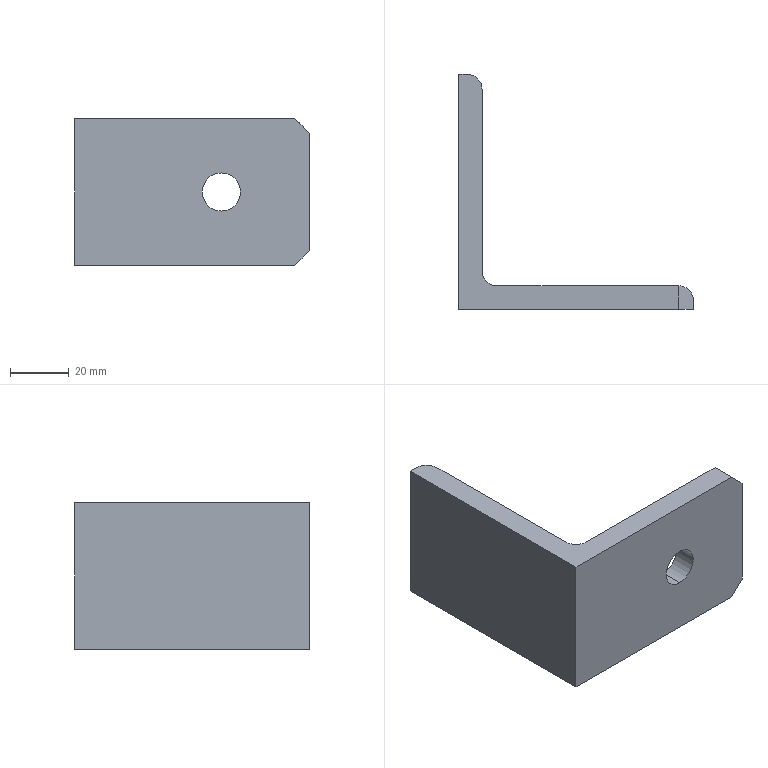Part | SolidWorks | features Fillet 3, Chamfer 1, Extrusion 1, ICE 1 | 1 solid | 15 faces | box 80 x 80 x 50 mm | volume 59312 mm3 | plane 10 | cylinder 5 | commonest cylinder face diameters 10 x3 13 x2
STEP:
#1=CARTESIAN_POINT('',(50.,-80.,18.5));
#2=VERTEX_POINT('',#1);
#3=CARTESIAN_POINT('',(50.,-80.,31.5));
#4=VERTEX_POINT('',#3);
#5=CARTESIAN_POINT('',(50.,-80.,25.));
#6=DIRECTION('',(0.,1.,0.));
#7=DIRECTION('',(0.,0.,1.));
#8=AXIS2_PLACEMENT_3D('',#5,#6,#7);
#9=CIRCLE('',#8,6.5);
#10=EDGE_CURVE('',#2,#4,#9,.T.);
#11=ORIENTED_EDGE('',*,*,#10,.F.);
#12=CARTESIAN_POINT('',(50.,-72.,18.5));
#13=VERTEX_POINT('',#12);
#14=CARTESIAN_POINT('',(50.,-122.,18.5));
#15=DIRECTION('',(0.,1.,0.));
#16=VECTOR('',#15,1000.);
#17=LINE('',#14,#16);
#18=EDGE_CURVE('',#2,#13,#17,.T.);
#19=ORIENTED_EDGE('',*,*,#18,.T.);
#20=CARTESIAN_POINT('',(50.,-72.,31.5));
#21=VERTEX_POINT('',#20);
#22=CARTESIAN_POINT('',(50.,-72.,25.));
#23=DIRECTION('',(0.,1.,0.));
#24=DIRECTION('',(0.,0.,1.));
#25=AXIS2_PLACEMENT_3D('',#22,#23,#24);
#26=CIRCLE('',#25,6.5);
#27=EDGE_CURVE('',#13,#21,#26,.T.);
#28=ORIENTED_EDGE('',*,*,#27,.T.);
#29=CARTESIAN_POINT('',(50.,-122.,31.5));
#30=DIRECTION('',(0.,1.,0.));
#31=VECTOR('',#30,1000.);
#32=LINE('',#29,#31);
#33=EDGE_CURVE('',#4,#21,#32,.T.);
#34=ORIENTED_EDGE('',*,*,#33,.F.);
#35=EDGE_LOOP('',(#11,#19,#28,#34));
#36=FACE_OUTER_BOUND('',#35,.T.);
#37=CARTESIAN_POINT('',(50.,-122.,25.));
#38=DIRECTION('',(0.,1.,0.));
#39=DIRECTION('',(0.,0.,1.));
#40=AXIS2_PLACEMENT_3D('',#37,#38,#39);
#41=CYLINDRICAL_SURFACE('',#40,6.5);
#42=ADVANCED_FACE('',(#36),#41,.F.);
#43=CARTESIAN_POINT('',(50.,-72.,25.));
#44=DIRECTION('',(0.,1.,0.));
#45=DIRECTION('',(0.,0.,1.));
#46=AXIS2_PLACEMENT_3D('',#43,#44,#45);
#47=CIRCLE('',#46,6.5);
#48=EDGE_CURVE('',#21,#13,#47,.T.);
#49=ORIENTED_EDGE('',*,*,#48,.F.);
#50=ORIENTED_EDGE('',*,*,#27,.F.);
#51=EDGE_LOOP('',(#49,#50));
#52=FACE_BOUND('',#51,.T.);
#53=CARTESIAN_POINT('',(13.,-72.,50.));
#54=VERTEX_POINT('',#53);
#55=CARTESIAN_POINT('',(75.,-72.,50.));
#56=VERTEX_POINT('',#55);
#57=CARTESIAN_POINT('',(8.,-72.,50.));
#58=DIRECTION('',(1.,0.,0.));
#59=VECTOR('',#58,1000.);
#60=LINE('',#57,#59);
#61=EDGE_CURVE('',#54,#56,#60,.T.);
#62=ORIENTED_EDGE('',*,*,#61,.T.);
#63=CARTESIAN_POINT('',(75.,-72.,0.));
#64=VERTEX_POINT('',#63);
#65=CARTESIAN_POINT('',(75.,-72.,50.));
#66=DIRECTION('',(0.,0.,-1.));
#67=VECTOR('',#66,1000.);
#68=LINE('',#65,#67);
#69=EDGE_CURVE('',#56,#64,#68,.T.);
#70=ORIENTED_EDGE('',*,*,#69,.T.);
#71=CARTESIAN_POINT('',(13.,-72.,0.));
#72=VERTEX_POINT('',#71);
#73=CARTESIAN_POINT('',(8.,-72.,0.));
#74=DIRECTION('',(1.,0.,0.));
#75=VECTOR('',#74,1000.);
#76=LINE('',#73,#75);
#77=EDGE_CURVE('',#72,#64,#76,.T.);
#78=ORIENTED_EDGE('',*,*,#77,.F.);
#79=CARTESIAN_POINT('',(13.,-72.,50.));
#80=DIRECTION('',(0.,0.,1.));
#81=VECTOR('',#80,1000.);
#82=LINE('',#79,#81);
#83=EDGE_CURVE('',#72,#54,#82,.T.);
#84=ORIENTED_EDGE('',*,*,#83,.T.);
#85=EDGE_LOOP('',(#62,#70,#78,#84));
#86=FACE_OUTER_BOUND('',#85,.T.);
#87=CARTESIAN_POINT('',(8.,-72.,50.));
#88=DIRECTION('',(0.,1.,0.));
#89=DIRECTION('',(0.,0.,1.));
#90=AXIS2_PLACEMENT_3D('',#87,#88,#89);
#91=PLANE('',#90);
#92=ADVANCED_FACE('',(#52,#86),#91,.T.);
#93=CARTESIAN_POINT('',(8.,-5.,0.));
#94=VERTEX_POINT('',#93);
#95=CARTESIAN_POINT('',(8.,-67.,0.));
#96=VERTEX_POINT('',#95);
#97=CARTESIAN_POINT('',(8.,0.,0.));
#98=DIRECTION('',(0.,-1.,0.));
#99=VECTOR('',#98,1000.);
#100=LINE('',#97,#99);
#101=EDGE_CURVE('',#94,#96,#100,.T.);
#102=ORIENTED_EDGE('',*,*,#101,.F.);
#103=CARTESIAN_POINT('',(8.,-5.,50.));
#104=VERTEX_POINT('',#103);
#105=CARTESIAN_POINT('',(8.,-5.,50.));
#106=DIRECTION('',(0.,0.,1.));
#107=VECTOR('',#106,1000.);
#108=LINE('',#105,#107);
#109=EDGE_CURVE('',#94,#104,#108,.T.);
#110=ORIENTED_EDGE('',*,*,#109,.T.);
#111=CARTESIAN_POINT('',(8.,-67.,50.));
#112=VERTEX_POINT('',#111);
#113=CARTESIAN_POINT('',(8.,0.,50.));
#114=DIRECTION('',(0.,-1.,0.));
#115=VECTOR('',#114,1000.);
#116=LINE('',#113,#115);
#117=EDGE_CURVE('',#104,#112,#116,.T.);
#118=ORIENTED_EDGE('',*,*,#117,.T.);
#119=CARTESIAN_POINT('',(8.,-67.,0.));
#120=DIRECTION('',(0.,0.,-1.));
#121=VECTOR('',#120,1000.);
#122=LINE('',#119,#121);
#123=EDGE_CURVE('',#112,#96,#122,.T.);
#124=ORIENTED_EDGE('',*,*,#123,.T.);
#125=EDGE_LOOP('',(#102,#110,#118,#124));
#126=FACE_OUTER_BOUND('',#125,.T.);
#127=CARTESIAN_POINT('',(8.,0.,50.));
#128=DIRECTION('',(1.,0.,0.));
#129=DIRECTION('',(0.,0.,-1.));
#130=AXIS2_PLACEMENT_3D('',#127,#128,#129);
#131=PLANE('',#130);
#132=ADVANCED_FACE('',(#126),#131,.T.);
#133=CARTESIAN_POINT('',(3.,0.,50.));
#134=VERTEX_POINT('',#133);
#135=CARTESIAN_POINT('',(0.,0.,50.));
#136=VERTEX_POINT('',#135);
#137=CARTESIAN_POINT('',(8.,0.,50.));
#138=DIRECTION('',(-1.,0.,0.));
#139=VECTOR('',#138,1000.);
#140=LINE('',#137,#139);
#141=EDGE_CURVE('',#134,#136,#140,.T.);
#142=ORIENTED_EDGE('',*,*,#141,.F.);
#143=CARTESIAN_POINT('',(3.,0.,0.));
#144=VERTEX_POINT('',#143);
#145=CARTESIAN_POINT('',(3.,0.,0.));
#146=DIRECTION('',(0.,0.,-1.));
#147=VECTOR('',#146,1000.);
#148=LINE('',#145,#147);
#149=EDGE_CURVE('',#134,#144,#148,.T.);
#150=ORIENTED_EDGE('',*,*,#149,.T.);
#151=CARTESIAN_POINT('',(0.,0.,0.));
#152=VERTEX_POINT('',#151);
#153=CARTESIAN_POINT('',(8.,0.,0.));
#154=DIRECTION('',(-1.,0.,0.));
#155=VECTOR('',#154,1000.);
#156=LINE('',#153,#155);
#157=EDGE_CURVE('',#144,#152,#156,.T.);
#158=ORIENTED_EDGE('',*,*,#157,.T.);
#159=CARTESIAN_POINT('',(0.,0.,50.));
#160=DIRECTION('',(0.,0.,-1.));
#161=VECTOR('',#160,1000.);
#162=LINE('',#159,#161);
#163=EDGE_CURVE('',#136,#152,#162,.T.);
#164=ORIENTED_EDGE('',*,*,#163,.F.);
#165=EDGE_LOOP('',(#142,#150,#158,#164));
#166=FACE_OUTER_BOUND('',#165,.T.);
#167=CARTESIAN_POINT('',(8.,0.,50.));
#168=DIRECTION('',(0.,-1.,0.));
#169=DIRECTION('',(0.,0.,-1.));
#170=AXIS2_PLACEMENT_3D('',#167,#168,#169);
#171=PLANE('',#170);
#172=ADVANCED_FACE('',(#166),#171,.F.);
#173=CARTESIAN_POINT('',(0.,-80.,0.));
#174=VERTEX_POINT('',#173);
#175=CARTESIAN_POINT('',(0.,0.,0.));
#176=DIRECTION('',(0.,-1.,0.));
#177=VECTOR('',#176,1000.);
#178=LINE('',#175,#177);
#179=EDGE_CURVE('',#152,#174,#178,.T.);
#180=ORIENTED_EDGE('',*,*,#179,.T.);
#181=CARTESIAN_POINT('',(0.,-80.,50.));
#182=VERTEX_POINT('',#181);
#183=CARTESIAN_POINT('',(0.,-80.,50.));
#184=DIRECTION('',(0.,0.,-1.));
#185=VECTOR('',#184,1000.);
#186=LINE('',#183,#185);
#187=EDGE_CURVE('',#182,#174,#186,.T.);
#188=ORIENTED_EDGE('',*,*,#187,.F.);
#189=CARTESIAN_POINT('',(0.,0.,50.));
#190=DIRECTION('',(0.,-1.,0.));
#191=VECTOR('',#190,1000.);
#192=LINE('',#189,#191);
#193=EDGE_CURVE('',#136,#182,#192,.T.);
#194=ORIENTED_EDGE('',*,*,#193,.F.);
#195=ORIENTED_EDGE('',*,*,#163,.T.);
#196=EDGE_LOOP('',(#180,#188,#194,#195));
#197=FACE_OUTER_BOUND('',#196,.T.);
#198=CARTESIAN_POINT('',(0.,0.,50.));
#199=DIRECTION('',(1.,0.,0.));
#200=DIRECTION('',(0.,0.,-1.));
#201=AXIS2_PLACEMENT_3D('',#198,#199,#200);
#202=PLANE('',#201);
#203=ADVANCED_FACE('',(#197),#202,.F.);
#204=CARTESIAN_POINT('',(50.,-80.,25.));
#205=DIRECTION('',(0.,1.,0.));
#206=DIRECTION('',(0.,0.,1.));
#207=AXIS2_PLACEMENT_3D('',#204,#205,#206);
#208=CIRCLE('',#207,6.5);
#209=EDGE_CURVE('',#4,#2,#208,.T.);
#210=ORIENTED_EDGE('',*,*,#209,.T.);
#211=ORIENTED_EDGE('',*,*,#10,.T.);
#212=EDGE_LOOP('',(#210,#211));
#213=FACE_BOUND('',#212,.T.);
#214=CARTESIAN_POINT('',(75.,-80.,0.));
#215=VERTEX_POINT('',#214);
#216=CARTESIAN_POINT('',(0.,-80.,0.));
#217=DIRECTION('',(1.,0.,0.));
#218=VECTOR('',#217,1000.);
#219=LINE('',#216,#218);
#220=EDGE_CURVE('',#174,#215,#219,.T.);
#221=ORIENTED_EDGE('',*,*,#220,.T.);
#222=CARTESIAN_POINT('',(80.,-80.,5.));
#223=VERTEX_POINT('',#222);
#224=CARTESIAN_POINT('',(75.,-80.,0.));
#225=DIRECTION('',(0.7071,0.,0.7071));
#226=VECTOR('',#225,1000.);
#227=LINE('',#224,#226);
#228=EDGE_CURVE('',#215,#223,#227,.T.);
#229=ORIENTED_EDGE('',*,*,#228,.T.);
#230=CARTESIAN_POINT('',(80.,-80.,45.));
#231=VERTEX_POINT('',#230);
#232=CARTESIAN_POINT('',(80.,-80.,50.));
#233=DIRECTION('',(0.,0.,-1.));
#234=VECTOR('',#233,1000.);
#235=LINE('',#232,#234);
#236=EDGE_CURVE('',#231,#223,#235,.T.);
#237=ORIENTED_EDGE('',*,*,#236,.F.);
#238=CARTESIAN_POINT('',(75.,-80.,50.));
#239=VERTEX_POINT('',#238);
#240=CARTESIAN_POINT('',(80.,-80.,45.));
#241=DIRECTION('',(-0.7071,0.,0.7071));
#242=VECTOR('',#241,1000.);
#243=LINE('',#240,#242);
#244=EDGE_CURVE('',#231,#239,#243,.T.);
#245=ORIENTED_EDGE('',*,*,#244,.T.);
#246=CARTESIAN_POINT('',(0.,-80.,50.));
#247=DIRECTION('',(1.,0.,0.));
#248=VECTOR('',#247,1000.);
#249=LINE('',#246,#248);
#250=EDGE_CURVE('',#182,#239,#249,.T.);
#251=ORIENTED_EDGE('',*,*,#250,.F.);
#252=ORIENTED_EDGE('',*,*,#187,.T.);
#253=EDGE_LOOP('',(#221,#229,#237,#245,#251,#252));
#254=FACE_OUTER_BOUND('',#253,.T.);
#255=CARTESIAN_POINT('',(0.,-80.,50.));
#256=DIRECTION('',(0.,1.,0.));
#257=DIRECTION('',(0.,0.,1.));
#258=AXIS2_PLACEMENT_3D('',#255,#256,#257);
#259=PLANE('',#258);
#260=ADVANCED_FACE('',(#213,#254),#259,.F.);
#261=CARTESIAN_POINT('',(80.,-77.,5.));
#262=VERTEX_POINT('',#261);
#263=CARTESIAN_POINT('',(80.,-72.,5.));
#264=DIRECTION('',(0.,1.,0.));
#265=VECTOR('',#264,1000.);
#266=LINE('',#263,#265);
#267=EDGE_CURVE('',#223,#262,#266,.T.);
#268=ORIENTED_EDGE('',*,*,#267,.T.);
#269=CARTESIAN_POINT('',(80.,-77.,45.));
#270=VERTEX_POINT('',#269);
#271=CARTESIAN_POINT('',(80.,-77.,50.));
#272=DIRECTION('',(0.,0.,1.));
#273=VECTOR('',#272,1000.);
#274=LINE('',#271,#273);
#275=EDGE_CURVE('',#262,#270,#274,.T.);
#276=ORIENTED_EDGE('',*,*,#275,.T.);
#277=CARTESIAN_POINT('',(80.,-80.,45.));
#278=DIRECTION('',(0.,-1.,0.));
#279=VECTOR('',#278,1000.);
#280=LINE('',#277,#279);
#281=EDGE_CURVE('',#270,#231,#280,.T.);
#282=ORIENTED_EDGE('',*,*,#281,.T.);
#283=ORIENTED_EDGE('',*,*,#236,.T.);
#284=EDGE_LOOP('',(#268,#276,#282,#283));
#285=FACE_OUTER_BOUND('',#284,.T.);
#286=CARTESIAN_POINT('',(80.,-72.,50.));
#287=DIRECTION('',(1.,0.,0.));
#288=DIRECTION('',(0.,0.,-1.));
#289=AXIS2_PLACEMENT_3D('',#286,#287,#288);
#290=PLANE('',#289);
#291=ADVANCED_FACE('',(#285),#290,.T.);
#292=ORIENTED_EDGE('',*,*,#250,.T.);
#293=CARTESIAN_POINT('',(75.,-72.,50.));
#294=DIRECTION('',(0.,1.,0.));
#295=VECTOR('',#294,1000.);
#296=LINE('',#293,#295);
#297=EDGE_CURVE('',#239,#56,#296,.T.);
#298=ORIENTED_EDGE('',*,*,#297,.T.);
#299=ORIENTED_EDGE('',*,*,#61,.F.);
#300=CARTESIAN_POINT('',(13.,-67.,50.));
#301=DIRECTION('',(0.,0.,-1.));
#302=DIRECTION('',(-1.,0.,0.));
#303=AXIS2_PLACEMENT_3D('',#300,#301,#302);
#304=CIRCLE('',#303,5.);
#305=EDGE_CURVE('',#54,#112,#304,.T.);
#306=ORIENTED_EDGE('',*,*,#305,.T.);
#307=ORIENTED_EDGE('',*,*,#117,.F.);
#308=CARTESIAN_POINT('',(3.,-5.,50.));
#309=DIRECTION('',(0.,0.,1.));
#310=DIRECTION('',(-1.,0.,0.));
#311=AXIS2_PLACEMENT_3D('',#308,#309,#310);
#312=CIRCLE('',#311,5.);
#313=EDGE_CURVE('',#104,#134,#312,.T.);
#314=ORIENTED_EDGE('',*,*,#313,.T.);
#315=ORIENTED_EDGE('',*,*,#141,.T.);
#316=ORIENTED_EDGE('',*,*,#193,.T.);
#317=EDGE_LOOP('',(#292,#298,#299,#306,#307,#314,#315,#316));
#318=FACE_OUTER_BOUND('',#317,.T.);
#319=CARTESIAN_POINT('',(0.,0.,50.));
#320=DIRECTION('',(0.,0.,-1.));
#321=DIRECTION('',(-1.,0.,0.));
#322=AXIS2_PLACEMENT_3D('',#319,#320,#321);
#323=PLANE('',#322);
#324=ADVANCED_FACE('',(#318),#323,.F.);
#325=ORIENTED_EDGE('',*,*,#77,.T.);
#326=CARTESIAN_POINT('',(75.,0.,0.));
#327=DIRECTION('',(0.,-1.,0.));
#328=VECTOR('',#327,1000.);
#329=LINE('',#326,#328);
#330=EDGE_CURVE('',#64,#215,#329,.T.);
#331=ORIENTED_EDGE('',*,*,#330,.T.);
#332=ORIENTED_EDGE('',*,*,#220,.F.);
#333=ORIENTED_EDGE('',*,*,#179,.F.);
#334=ORIENTED_EDGE('',*,*,#157,.F.);
#335=CARTESIAN_POINT('',(3.,-5.,0.));
#336=DIRECTION('',(0.,0.,-1.));
#337=DIRECTION('',(-1.,0.,0.));
#338=AXIS2_PLACEMENT_3D('',#335,#336,#337);
#339=CIRCLE('',#338,5.);
#340=EDGE_CURVE('',#144,#94,#339,.T.);
#341=ORIENTED_EDGE('',*,*,#340,.T.);
#342=ORIENTED_EDGE('',*,*,#101,.T.);
#343=CARTESIAN_POINT('',(13.,-67.,0.));
#344=DIRECTION('',(0.,0.,1.));
#345=DIRECTION('',(-1.,0.,0.));
#346=AXIS2_PLACEMENT_3D('',#343,#344,#345);
#347=CIRCLE('',#346,5.);
#348=EDGE_CURVE('',#96,#72,#347,.T.);
#349=ORIENTED_EDGE('',*,*,#348,.T.);
#350=EDGE_LOOP('',(#325,#331,#332,#333,#334,#341,#342,#349));
#351=FACE_OUTER_BOUND('',#350,.T.);
#352=CARTESIAN_POINT('',(0.,0.,0.));
#353=DIRECTION('',(0.,0.,-1.));
#354=DIRECTION('',(-1.,0.,0.));
#355=AXIS2_PLACEMENT_3D('',#352,#353,#354);
#356=PLANE('',#355);
#357=ADVANCED_FACE('',(#351),#356,.T.);
#358=ORIENTED_EDGE('',*,*,#18,.F.);
#359=ORIENTED_EDGE('',*,*,#209,.F.);
#360=ORIENTED_EDGE('',*,*,#33,.T.);
#361=ORIENTED_EDGE('',*,*,#48,.T.);
#362=EDGE_LOOP('',(#358,#359,#360,#361));
#363=FACE_OUTER_BOUND('',#362,.T.);
#364=CARTESIAN_POINT('',(50.,-122.,25.));
#365=DIRECTION('',(0.,1.,0.));
#366=DIRECTION('',(0.,0.,1.));
#367=AXIS2_PLACEMENT_3D('',#364,#365,#366);
#368=CYLINDRICAL_SURFACE('',#367,6.5);
#369=ADVANCED_FACE('',(#363),#368,.F.);
#370=ORIENTED_EDGE('',*,*,#305,.F.);
#371=ORIENTED_EDGE('',*,*,#83,.F.);
#372=ORIENTED_EDGE('',*,*,#348,.F.);
#373=ORIENTED_EDGE('',*,*,#123,.F.);
#374=EDGE_LOOP('',(#370,#371,#372,#373));
#375=FACE_OUTER_BOUND('',#374,.T.);
#376=CARTESIAN_POINT('',(13.,-67.,50.));
#377=DIRECTION('',(0.,0.,1.));
#378=DIRECTION('',(1.,0.,0.));
#379=AXIS2_PLACEMENT_3D('',#376,#377,#378);
#380=CYLINDRICAL_SURFACE('',#379,5.);
#381=ADVANCED_FACE('',(#375),#380,.F.);
#382=ORIENTED_EDGE('',*,*,#313,.F.);
#383=ORIENTED_EDGE('',*,*,#109,.F.);
#384=ORIENTED_EDGE('',*,*,#340,.F.);
#385=ORIENTED_EDGE('',*,*,#149,.F.);
#386=EDGE_LOOP('',(#382,#383,#384,#385));
#387=FACE_OUTER_BOUND('',#386,.T.);
#388=CARTESIAN_POINT('',(3.,-5.,50.));
#389=DIRECTION('',(0.,0.,1.));
#390=DIRECTION('',(1.,0.,0.));
#391=AXIS2_PLACEMENT_3D('',#388,#389,#390);
#392=CYLINDRICAL_SURFACE('',#391,5.);
#393=ADVANCED_FACE('',(#387),#392,.T.);
#394=ORIENTED_EDGE('',*,*,#330,.F.);
#395=CARTESIAN_POINT('',(75.,-72.,0.));
#396=CARTESIAN_POINT('',(77.929,-72.,2.929));
#397=CARTESIAN_POINT('',(80.,-74.071,5.));
#398=CARTESIAN_POINT('',(80.,-77.,5.));
#399=(BOUNDED_CURVE()B_SPLINE_CURVE(3,(#395,#396,#397,#398),.UNSPECIFIED.,.F.,.F.)B_SPLINE_CURVE_WITH_KNOTS((4,4),(1.571,3.142),.UNSPECIFIED.)CURVE()GEOMETRIC_REPRESENTATION_ITEM()RATIONAL_B_SPLINE_CURVE((1.,0.8047,0.8047,1.))REPRESENTATION_ITEM(''));
#400=EDGE_CURVE('',#64,#262,#399,.T.);
#401=ORIENTED_EDGE('',*,*,#400,.T.);
#402=ORIENTED_EDGE('',*,*,#267,.F.);
#403=ORIENTED_EDGE('',*,*,#228,.F.);
#404=EDGE_LOOP('',(#394,#401,#402,#403));
#405=FACE_OUTER_BOUND('',#404,.T.);
#406=CARTESIAN_POINT('',(75.,0.,0.));
#407=DIRECTION('',(-0.7071,0.,0.7071));
#408=DIRECTION('',(0.,-1.,0.));
#409=AXIS2_PLACEMENT_3D('',#406,#407,#408);
#410=PLANE('',#409);
#411=ADVANCED_FACE('',(#405),#410,.F.);
#412=ORIENTED_EDGE('',*,*,#281,.F.);
#413=CARTESIAN_POINT('',(80.,-77.,45.));
#414=CARTESIAN_POINT('',(80.,-74.071,45.));
#415=CARTESIAN_POINT('',(77.929,-72.,47.071));
#416=CARTESIAN_POINT('',(75.,-72.,50.));
#417=(BOUNDED_CURVE()B_SPLINE_CURVE(3,(#413,#414,#415,#416),.UNSPECIFIED.,.F.,.F.)B_SPLINE_CURVE_WITH_KNOTS((4,4),(0.,1.571),.UNSPECIFIED.)CURVE()GEOMETRIC_REPRESENTATION_ITEM()RATIONAL_B_SPLINE_CURVE((1.,0.8047,0.8047,1.))REPRESENTATION_ITEM(''));
#418=EDGE_CURVE('',#270,#56,#417,.T.);
#419=ORIENTED_EDGE('',*,*,#418,.T.);
#420=ORIENTED_EDGE('',*,*,#297,.F.);
#421=ORIENTED_EDGE('',*,*,#244,.F.);
#422=EDGE_LOOP('',(#412,#419,#420,#421));
#423=FACE_OUTER_BOUND('',#422,.T.);
#424=CARTESIAN_POINT('',(80.,-72.,45.));
#425=DIRECTION('',(0.7071,0.,0.7071));
#426=DIRECTION('',(0.,1.,0.));
#427=AXIS2_PLACEMENT_3D('',#424,#425,#426);
#428=PLANE('',#427);
#429=ADVANCED_FACE('',(#423),#428,.T.);
#430=ORIENTED_EDGE('',*,*,#418,.F.);
#431=ORIENTED_EDGE('',*,*,#275,.F.);
#432=ORIENTED_EDGE('',*,*,#400,.F.);
#433=ORIENTED_EDGE('',*,*,#69,.F.);
#434=EDGE_LOOP('',(#430,#431,#432,#433));
#435=FACE_OUTER_BOUND('',#434,.T.);
#436=CARTESIAN_POINT('',(75.,-77.,50.));
#437=DIRECTION('',(0.,0.,-1.));
#438=DIRECTION('',(-1.,0.,0.));
#439=AXIS2_PLACEMENT_3D('',#436,#437,#438);
#440=CYLINDRICAL_SURFACE('',#439,5.);
#441=ADVANCED_FACE('',(#435),#440,.T.);
#442=CLOSED_SHELL('',(#42,#92,#132,#172,#203,#260,#291,#324,#357,#369,#381,#393,#411,#429,#441));
#443=MANIFOLD_SOLID_BREP('',#442);
#444=CARTESIAN_POINT('',(0.,0.,0.));
#445=DIRECTION('',(0.,0.,1.));
#446=DIRECTION('',(1.,0.,0.));
#447=AXIS2_PLACEMENT_3D('',#444,#445,#446);
#448=(LENGTH_UNIT()NAMED_UNIT(*)SI_UNIT(.MILLI.,.METRE.));
#449=UNCERTAINTY_MEASURE_WITH_UNIT(LENGTH_MEASURE(0.00001),#448,'','');
#450=(NAMED_UNIT(*)PLANE_ANGLE_UNIT()SI_UNIT($,.RADIAN.));
#451=(NAMED_UNIT(*)SI_UNIT($,.STERADIAN.)SOLID_ANGLE_UNIT());
#452=(GEOMETRIC_REPRESENTATION_CONTEXT(3)GLOBAL_UNCERTAINTY_ASSIGNED_CONTEXT((#449))GLOBAL_UNIT_ASSIGNED_CONTEXT((#448,#450,#451))REPRESENTATION_CONTEXT('',''));
#453=ADVANCED_BREP_SHAPE_REPRESENTATION('',(#443,#447),#452);